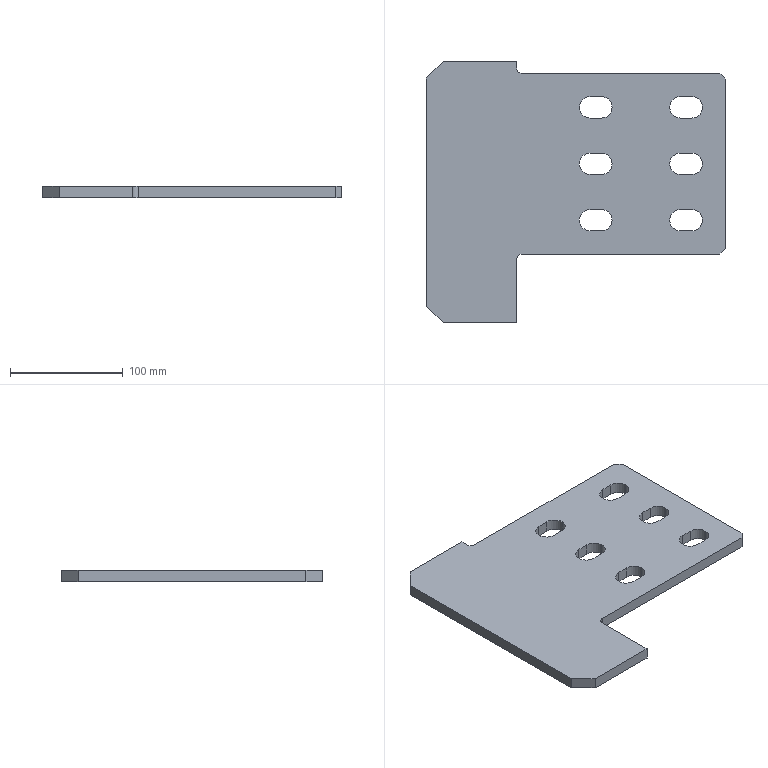Part | STEP file | 筋Plate-250×125-200-30度 | 1 solid | 46 faces | box 265 x 232 x 10 mm | volume 450796 mm3 | plane 26 | cylinder 20 | commonest cylinder face diameters 19 x18 10 x2